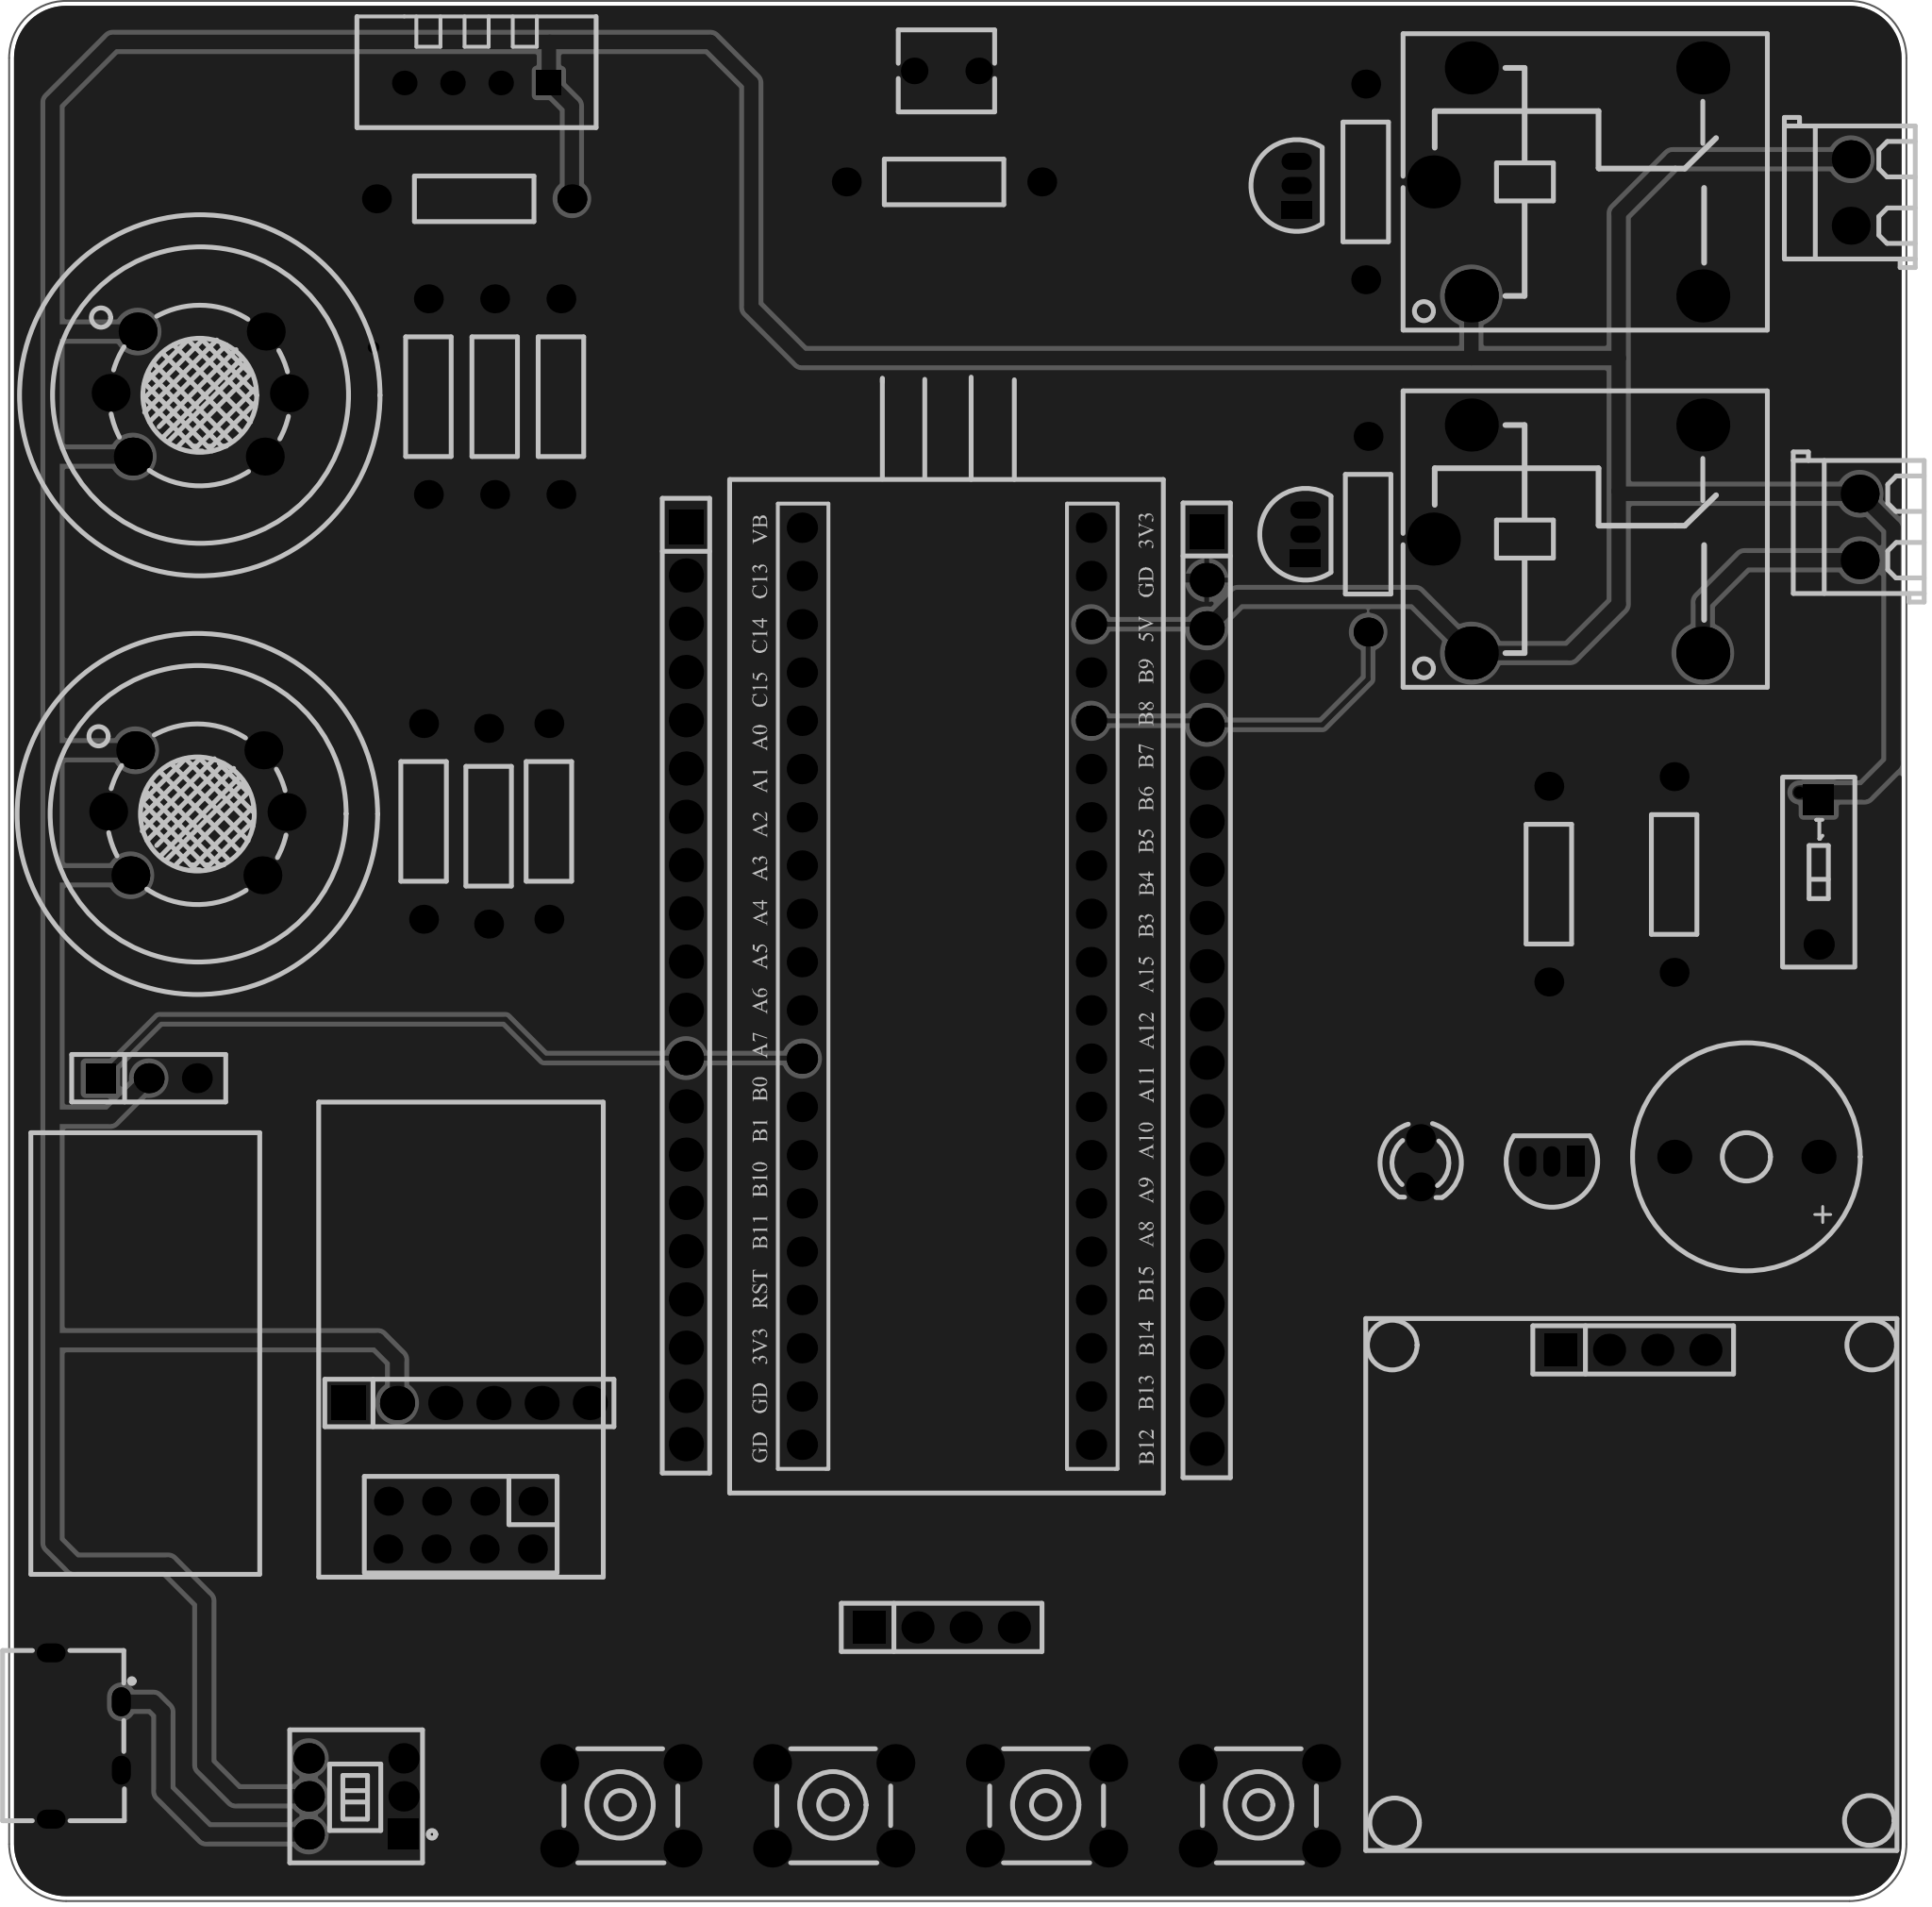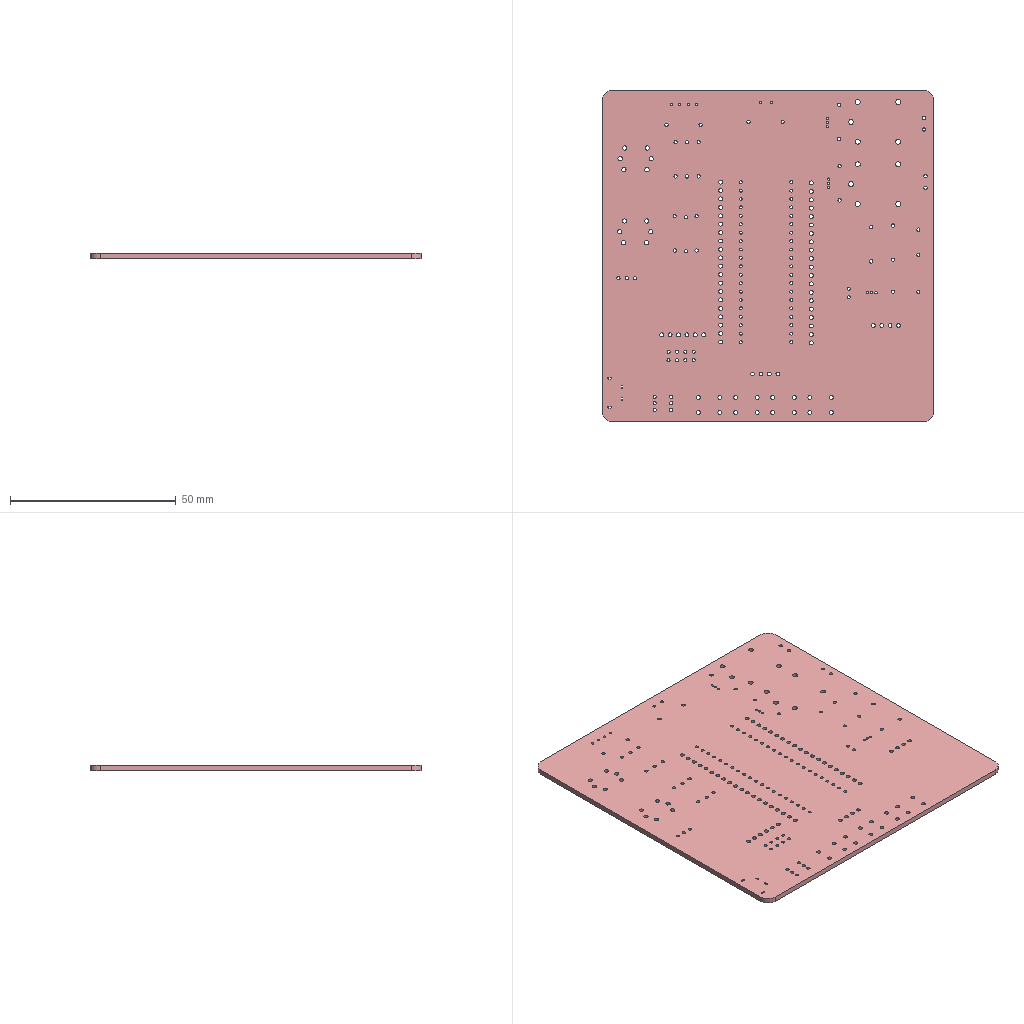Circuit board layout | Altium Designer | box 100 x 100 x 1.6 mm
Layer stack:
# Altium Designer layer stack of  (unit mm; dielectric type: 0 none, 1 core, 2 prepreg, 3 surface material)
index,name,kind,layer,copper_thickness_mm,dielectric_type,dielectric_thickness_mm,dielectric_material,dielectric_constant
0,Top Paste Mask Layer,other,,,,,,
1,Top Silkscreen Layer,other,,,,,,
2,Top Solder Mask Layer,dielectric,,,3,0.01,,3.3
3,Top Layer,copper,Top Layer,0.035,,,,
4,Dielectric1,dielectric,,,3,1.51,FR4,4.5
5,Bottom Layer,copper,Bottom Layer,0.035,,,,
6,Bottom Solder Mask Layer,dielectric,,,3,0.01,,3.3
7,Bottom Silkscreen Layer,other,,,,,,
8,Bottom Paste Mask Layer,other,,,,,,
# drill layer pairs: low layer,high layer
drill_pair,Top Layer,Bottom Layer
Part placement:
Designator,Comment,Layer,Footprint,Center-X(mm),Center-Y(mm),Rotation
H3,,TopLayer,HDR-TH_20P-P2.54-V-F,146.812,132.588,270
H4,,TopLayer,HDR-TH_20P-P2.54-V-F,119.366,132.831,270
H6,,TopLayer,HDR-TH_3P-P2.54-V-F,91.048,127.962,0
H7,,TopLayer,HDR-TH_4P-P2.54-V-F,132.842,99.06,0
R7,1kΩ,TopLayer,Res_1/4W,132.969,175.133,180
SW5,NDS-01V,TopLayer,SW-TH_2P-L3.9-W9.9-P2.54-LS7.6,179.07,138.811,270
U1,MQ-2,TopLayer,SENSOR-TH_MQ-2,93.614,141.932,0
U3,光敏电阻-5MM,TopLayer,RES-TH_L4.9-W4.3-P3.4,133.096,180.975,180
U7,DHT11,TopLayer,SENSOR-TH_DHT11,108.331,180.34,180
BUZZER1,2.3kHz,TopLayer,BUZ-TH_BD12.0-P7.60-D0.6-FD,175.26,123.825,180
H10,2.54-1*4P female,TopLayer,HDR-TH_4P-P2.54-V-F,169.291,113.665,0
H13,,TopLayer,HDR-TH_6P-P2.54-V-M-1,107.95,110.871,0
KEY1,Button 1,TopLayer,KEY-TH_4P-L6.0-W6.0-P4.50-LS7.5,115.937,89.672,0
KEY3,Button 2,TopLayer,KEY-TH_4P-L6.0-W6.0-P4.50-LS7.5,138.374,89.672,0
KEY4,Button 4,TopLayer,KEY-TH_4P-L6.0-W6.0-P4.50-LS7.5,149.592,89.672,0
KEY5,Button 5,TopLayer,KEY-TH_4P-L6.0-W6.0-P4.50-LS7.5,127.156,89.672,0
Q1,,TopLayer,S8050_TO_92,165.006,123.586,180
R8,1kΩ,TopLayer,Res_1/4W,171.45,138.684,270
R9,120,TopLayer,Res_1/4W,164.846,138.176,270
SW8,TK-6700-1,TopLayer,SW-TH_TK-6700-1,101.981,90.17,90
U2,MQ-5,TopLayer,SENSOR-TH_MQ-2,93.741,163.967,0
U44,,TopLayer,STM32最小系统板,133.098,132.803,0
U98,,TopLayer,WiFi封装,107.479,104.445,0
USB1,KH-TYPE-C-2P,TopLayer,USB-SMD_KH-TYPE-C-2P,87.757,93.345,270
Q2,,TopLayer,S8050_TO_92,151.556,174.944,90
R1,10kΩ,TopLayer,Res_1/4W,108.966,141.224,90
R2,10kΩ,TopLayer,Res_1/4W,112.141,141.478,90
R3,5Ω,TopLayer,Res_1/4W,105.537,141.478,90
R4,10kΩ,TopLayer,Res_1/4W,109.284,163.83,90
R5,10kΩ,TopLayer,Res_1/4W,112.776,163.83,90
R6,5Ω,TopLayer,Res_1/4W,105.791,163.83,90
R13,10kΩ,TopLayer,Res_1/4W,108.204,174.244,0
R15,1kΩ,TopLayer,Res_1/4W,155.194,175.133,90
RLY1,SRD-05VDC-SL-C,TopLayer,RELAY-TH_SRD-XXVDC-XL-C,165.862,175.133,0
U4,KF350-3.5-2P,TopLayer,CONN-TH_P3.50_KF350-3.5-2P,180.759,174.577,90
Q3,,TopLayer,S8050_TO_92,152.019,156.591,90
R10,1kΩ,TopLayer,Res_1/4W,155.321,156.591,90
RLY2,SRD-05VDC-SL-C,TopLayer,RELAY-TH_SRD-XXVDC-XL-C,165.862,156.337,0
U5,KF350-3.5-2P,TopLayer,CONN-TH_P3.50_KF350-3.5-2P,181.229,156.972,90
LED1,,TopLayer,LED_TH-3mm,158.077,123.513,270
Pad and via stacks:
# Altium Designer via and pad stacks of  (unit mm). Each distinct definition once, with the count of objects using it.
# via: kind,start_layer,end_layer,hole_mm,diameter_mm,mode(0 simple;1 top-mid-bottom;2 full stack),diameter_per_layer,count,example_net
# pad: kind,layer,hole_mm,hole_type(0 round;1 square;2 slot),plating,top_size,top_shape(1 round;2 rect;3 octagon;9 rounded rect),mid_size,bottom_size,mode,footprint,size_per_layer,count,example
pad,Multi-Layer,1.2,0,plated,1.8x1.8,2,1.8x1.8,1.8x1.8,0,HDR-TH_20P-P2.54-V-F,,2,H3.1
pad,Multi-Layer,1.2,0,plated,1.8x1.8,1,1.8x1.8,1.8x1.8,0,HDR-TH_20P-P2.54-V-F,,38,H3.2
pad,Multi-Layer,1.02,0,plated,1.575x1.575,1,1.575x1.575,1.575x1.575,0,HDR-TH_3P-P2.54-V-F,,2,H6.3
pad,Multi-Layer,1.02,0,plated,1.575x1.575,2,1.575x1.575,1.575x1.575,0,HDR-TH_3P-P2.54-V-F,,1,H6.1
pad,Multi-Layer,1.1,0,plated,1.7x1.7,2,1.7x1.7,1.7x1.7,0,HDR-TH_4P-P2.54-V-F,,2,H7.1
pad,Multi-Layer,1.1,0,plated,1.7x1.7,1,1.7x1.7,1.7x1.7,0,HDR-TH_4P-P2.54-V-F,,6,H7.2
pad,Multi-Layer,1,0,plated,1.524x1.524,1,1.524x1.524,1.524x1.524,0,Res_1/4W,,24,R7.1
pad,Multi-Layer,1,0,plated,1.6x1.6,2,1.6x1.6,1.6x1.6,0,SW-TH_2P-L3.9-W9.9-P2.54-LS7.6,,1,SW5.1
pad,Multi-Layer,1,0,plated,1.6x1.6,1,1.6x1.6,1.6x1.6,0,SW-TH_2P-L3.9-W9.9-P2.54-LS7.6,,1,SW5.2
pad,Multi-Layer,1.3,0,plated,2x2,1,2x2,2x2,0,SENSOR-TH_MQ-2,,12,U1.1
pad,Multi-Layer,0.8,0,plated,1.4x1.4,1,1.4x1.4,1.4x1.4,0,RES-TH_L4.9-W4.3-P3.4,,2,U3.1
pad,Multi-Layer,0.7112,0,plated,1.295x1.295,2,1.295x1.295,1.295x1.295,0,SENSOR-TH_DHT11,,1,U7.1
pad,Multi-Layer,0.7112,0,plated,1.295x1.295,1,1.295x1.295,1.295x1.295,0,SENSOR-TH_DHT11,,3,U7.2
pad,Multi-Layer,1,0,plated,1.8x1.8,1,1.8x1.8,1.8x1.8,0,BUZ-TH_BD12.0-P7.60-D0.6-FD,,2,BUZZER1.2
pad,Multi-Layer,1.2,0,plated,1.8x1.8,1,1.8x1.8,1.8x1.8,0,HDR-TH_6P-P2.54-V-M-1,,5,H13.6
pad,Multi-Layer,1.2,0,plated,1.8x1.8,2,1.8x1.8,1.8x1.8,0,HDR-TH_6P-P2.54-V-M-1,,1,H13.1
pad,Multi-Layer,1.2,0,plated,2x2,1,2x2,2x2,0,KEY-TH_4P-L6.0-W6.0-P4.50-LS7.5,,16,KEY1.1
pad,Multi-Layer,0.701,0,plated,0.8992x1.6,2,0.8992x1.6,0.8992x1.6,0,S8050_TO_92,,3,Q1.1
pad,Multi-Layer,0.701,0,plated,0.8992x1.6,1,0.8992x1.6,0.8992x1.6,0,S8050_TO_92,,6,Q1.2
pad,Multi-Layer,1,0,plated,1.6x1.6,2,1.6x1.6,1.6x1.6,0,SW-TH_TK-6700-1,,1,SW8.1
pad,Multi-Layer,1,0,plated,1.6x1.6,1,1.6x1.6,1.6x1.6,0,SW-TH_TK-6700-1,,5,SW8.2
pad,Multi-Layer,0.9,0,plated,1.6x1.6,1,1.6x1.6,1.6x1.6,0,STM32\u00D7\u00EE\u00D0\u00A1\u00CF\u00B5\u00CD\u00B3\u00B0\u00E5,,40,U44.40
pad,Multi-Layer,0.9144,0,plated,1.524x1.524,1,1.524x1.524,1.524x1.524,0,WiFi\u00B7\u00E2\u00D7\u00B0,,8,U98.1
pad,Multi-Layer,0.45,2,plated,1x1.524,1,1x1.524,1x1.524,0,USB-SMD_KH-TYPE-C-2P,,2,USB1.1
pad,Multi-Layer,0.5,2,plated,1x1.524,1,1x1.524,1x1.524,0,USB-SMD_KH-TYPE-C-2P,,2,USB1.3
pad,Multi-Layer,1.524,0,plated,2.794x2.794,1,2.794x2.794,2.794x2.794,0,RELAY-TH_SRD-XXVDC-XL-C,,10,RLY1.2
pad,Multi-Layer,1,0,plated,2x2,1,2x2,2x2,0,CONN-TH_P3.50_KF350-3.5-2P,,4,U4.1
pad,Multi-Layer,0.9144,0,plated,1.524x1.524,1,1.524x1.524,1.524x1.524,0,LED_TH-3mm,,2,LED1.1
via,Top Layer,Bottom Layer,0.3048,0.61,0,,2,+5V
Copper pours:
name,layer,net,type(0 solid;1 hatched;2 none)
Bottom Layer-GND,Bottom Layer,GND,0
Top Layer-GND,Top Layer,GND,0
Design rules, without the lines most boards share:
# Altium Designer design rules of  (exported by Altium Designer, unit mm)
# columns: name | kind | enabled | priority | scope1 | scope2 | descriptor | typed fields (field=value)
creepage | 65 | enabled | 1 | All | All | Creepage Distance Constraint =(0mil) (All),(All) |